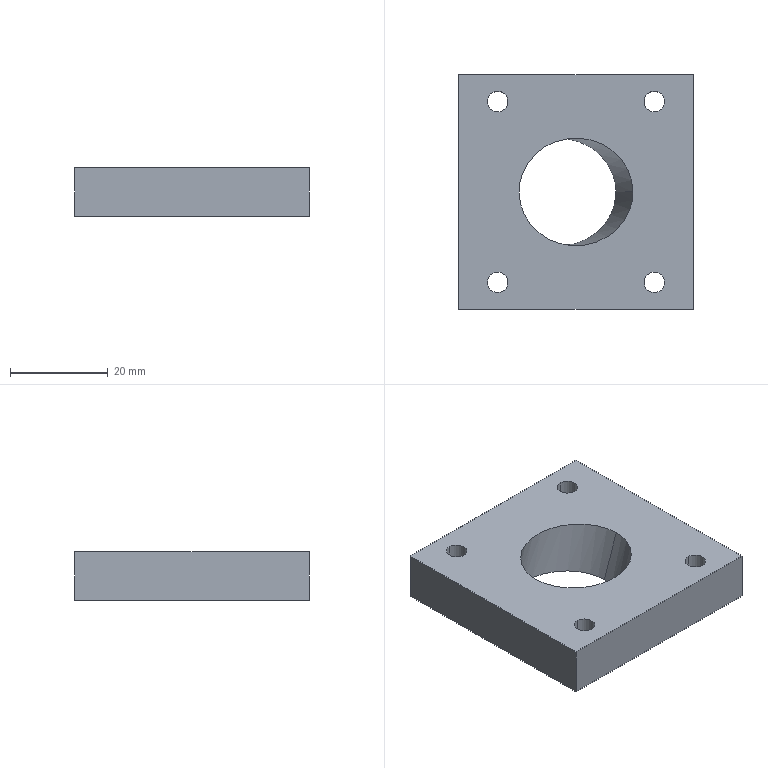Part | SolidWorks | features BaseBody 1 | 1 solid | 16 faces | box 48 x 48 x 10 mm | volume 18462 mm3 | cylinder 10 | plane 6 | commonest cylinder face diameters 4.2 x8 22 x2
STEP:
#1=CARTESIAN_POINT('',(-11.643,0.,10.));
#2=VERTEX_POINT('',#1);
#3=CARTESIAN_POINT('',(11.643,0.,10.));
#4=VERTEX_POINT('',#3);
#5=CARTESIAN_POINT('',(-11.643,0.,10.));
#6=CARTESIAN_POINT('',(-11.643,-22.,10.));
#7=CARTESIAN_POINT('',(11.643,-22.,10.));
#8=CARTESIAN_POINT('',(11.643,0.,10.));
#9=(BOUNDED_CURVE()B_SPLINE_CURVE(3,(#5,#6,#7,#8),.UNSPECIFIED.,.F.,.F.)B_SPLINE_CURVE_WITH_KNOTS((4,4),(0.,3.142),.UNSPECIFIED.)CURVE()GEOMETRIC_REPRESENTATION_ITEM()RATIONAL_B_SPLINE_CURVE((1.,0.3333,0.3333,1.))REPRESENTATION_ITEM(''));
#10=EDGE_CURVE('',#2,#4,#9,.T.);
#11=ORIENTED_EDGE('',*,*,#10,.T.);
#12=CARTESIAN_POINT('',(8.174,0.,0.));
#13=VERTEX_POINT('',#12);
#14=CARTESIAN_POINT('',(11.679,0.,10.103));
#15=DIRECTION('',(-0.3277,0.,-0.9448));
#16=VECTOR('',#15,1000.);
#17=LINE('',#14,#16);
#18=EDGE_CURVE('',#4,#13,#17,.T.);
#19=ORIENTED_EDGE('',*,*,#18,.T.);
#20=CARTESIAN_POINT('',(-15.112,0.,0.));
#21=VERTEX_POINT('',#20);
#22=CARTESIAN_POINT('',(8.174,0.,0.));
#23=CARTESIAN_POINT('',(8.174,-22.,0.));
#24=CARTESIAN_POINT('',(-15.112,-22.,0.));
#25=CARTESIAN_POINT('',(-15.112,0.,0.));
#26=(BOUNDED_CURVE()B_SPLINE_CURVE(3,(#22,#23,#24,#25),.UNSPECIFIED.,.F.,.F.)B_SPLINE_CURVE_WITH_KNOTS((4,4),(3.142,6.283),.UNSPECIFIED.)CURVE()GEOMETRIC_REPRESENTATION_ITEM()RATIONAL_B_SPLINE_CURVE((1.,0.3333,0.3333,1.))REPRESENTATION_ITEM(''));
#27=EDGE_CURVE('',#13,#21,#26,.T.);
#28=ORIENTED_EDGE('',*,*,#27,.T.);
#29=CARTESIAN_POINT('',(-9.106,0.,17.313));
#30=DIRECTION('',(-0.3277,0.,-0.9448));
#31=VECTOR('',#30,1000.);
#32=LINE('',#29,#31);
#33=EDGE_CURVE('',#2,#21,#32,.T.);
#34=ORIENTED_EDGE('',*,*,#33,.F.);
#35=EDGE_LOOP('',(#11,#19,#28,#34));
#36=FACE_OUTER_BOUND('',#35,.T.);
#37=CARTESIAN_POINT('',(1.286,0.,13.708));
#38=DIRECTION('',(-0.3277,0.,-0.9448));
#39=DIRECTION('',(-0.9448,0.,0.3277));
#40=AXIS2_PLACEMENT_3D('',#37,#38,#39);
#41=CYLINDRICAL_SURFACE('',#40,11.);
#42=ADVANCED_FACE('',(#36),#41,.F.);
#43=CARTESIAN_POINT('',(16.,20.6,10.));
#44=VERTEX_POINT('',#43);
#45=CARTESIAN_POINT('',(16.,16.4,10.));
#46=VERTEX_POINT('',#45);
#47=CARTESIAN_POINT('',(16.,18.5,10.));
#48=DIRECTION('',(0.,0.,1.));
#49=DIRECTION('',(0.,1.,0.));
#50=AXIS2_PLACEMENT_3D('',#47,#48,#49);
#51=CIRCLE('',#50,2.1);
#52=EDGE_CURVE('',#44,#46,#51,.T.);
#53=ORIENTED_EDGE('',*,*,#52,.T.);
#54=CARTESIAN_POINT('',(16.,16.4,0.));
#55=VERTEX_POINT('',#54);
#56=CARTESIAN_POINT('',(16.,16.4,10.));
#57=DIRECTION('',(0.,0.,-1.));
#58=VECTOR('',#57,1000.);
#59=LINE('',#56,#58);
#60=EDGE_CURVE('',#46,#55,#59,.T.);
#61=ORIENTED_EDGE('',*,*,#60,.T.);
#62=CARTESIAN_POINT('',(16.,20.6,0.));
#63=VERTEX_POINT('',#62);
#64=CARTESIAN_POINT('',(16.,18.5,0.));
#65=DIRECTION('',(0.,0.,1.));
#66=DIRECTION('',(0.,1.,0.));
#67=AXIS2_PLACEMENT_3D('',#64,#65,#66);
#68=CIRCLE('',#67,2.1);
#69=EDGE_CURVE('',#63,#55,#68,.T.);
#70=ORIENTED_EDGE('',*,*,#69,.F.);
#71=CARTESIAN_POINT('',(16.,20.6,10.));
#72=DIRECTION('',(0.,0.,-1.));
#73=VECTOR('',#72,1000.);
#74=LINE('',#71,#73);
#75=EDGE_CURVE('',#44,#63,#74,.T.);
#76=ORIENTED_EDGE('',*,*,#75,.F.);
#77=EDGE_LOOP('',(#53,#61,#70,#76));
#78=FACE_OUTER_BOUND('',#77,.T.);
#79=CARTESIAN_POINT('',(16.,18.5,10.));
#80=DIRECTION('',(0.,0.,-1.));
#81=DIRECTION('',(0.,1.,0.));
#82=AXIS2_PLACEMENT_3D('',#79,#80,#81);
#83=CYLINDRICAL_SURFACE('',#82,2.1);
#84=ADVANCED_FACE('',(#78),#83,.F.);
#85=CARTESIAN_POINT('',(-16.,-16.4,10.));
#86=VERTEX_POINT('',#85);
#87=CARTESIAN_POINT('',(-16.,-20.6,10.));
#88=VERTEX_POINT('',#87);
#89=CARTESIAN_POINT('',(-16.,-18.5,10.));
#90=DIRECTION('',(0.,0.,1.));
#91=DIRECTION('',(0.,1.,0.));
#92=AXIS2_PLACEMENT_3D('',#89,#90,#91);
#93=CIRCLE('',#92,2.1);
#94=EDGE_CURVE('',#86,#88,#93,.T.);
#95=ORIENTED_EDGE('',*,*,#94,.T.);
#96=CARTESIAN_POINT('',(-16.,-20.6,0.));
#97=VERTEX_POINT('',#96);
#98=CARTESIAN_POINT('',(-16.,-20.6,10.));
#99=DIRECTION('',(0.,0.,-1.));
#100=VECTOR('',#99,1000.);
#101=LINE('',#98,#100);
#102=EDGE_CURVE('',#88,#97,#101,.T.);
#103=ORIENTED_EDGE('',*,*,#102,.T.);
#104=CARTESIAN_POINT('',(-16.,-16.4,0.));
#105=VERTEX_POINT('',#104);
#106=CARTESIAN_POINT('',(-16.,-18.5,0.));
#107=DIRECTION('',(0.,0.,1.));
#108=DIRECTION('',(0.,1.,0.));
#109=AXIS2_PLACEMENT_3D('',#106,#107,#108);
#110=CIRCLE('',#109,2.1);
#111=EDGE_CURVE('',#105,#97,#110,.T.);
#112=ORIENTED_EDGE('',*,*,#111,.F.);
#113=CARTESIAN_POINT('',(-16.,-16.4,10.));
#114=DIRECTION('',(0.,0.,-1.));
#115=VECTOR('',#114,1000.);
#116=LINE('',#113,#115);
#117=EDGE_CURVE('',#86,#105,#116,.T.);
#118=ORIENTED_EDGE('',*,*,#117,.F.);
#119=EDGE_LOOP('',(#95,#103,#112,#118));
#120=FACE_OUTER_BOUND('',#119,.T.);
#121=CARTESIAN_POINT('',(-16.,-18.5,10.));
#122=DIRECTION('',(0.,0.,-1.));
#123=DIRECTION('',(0.,1.,0.));
#124=AXIS2_PLACEMENT_3D('',#121,#122,#123);
#125=CYLINDRICAL_SURFACE('',#124,2.1);
#126=ADVANCED_FACE('',(#120),#125,.F.);
#127=CARTESIAN_POINT('',(-16.,20.6,10.));
#128=VERTEX_POINT('',#127);
#129=CARTESIAN_POINT('',(-16.,16.4,10.));
#130=VERTEX_POINT('',#129);
#131=CARTESIAN_POINT('',(-16.,18.5,10.));
#132=DIRECTION('',(0.,0.,1.));
#133=DIRECTION('',(0.,1.,0.));
#134=AXIS2_PLACEMENT_3D('',#131,#132,#133);
#135=CIRCLE('',#134,2.1);
#136=EDGE_CURVE('',#128,#130,#135,.T.);
#137=ORIENTED_EDGE('',*,*,#136,.T.);
#138=CARTESIAN_POINT('',(-16.,16.4,0.));
#139=VERTEX_POINT('',#138);
#140=CARTESIAN_POINT('',(-16.,16.4,10.));
#141=DIRECTION('',(0.,0.,-1.));
#142=VECTOR('',#141,1000.);
#143=LINE('',#140,#142);
#144=EDGE_CURVE('',#130,#139,#143,.T.);
#145=ORIENTED_EDGE('',*,*,#144,.T.);
#146=CARTESIAN_POINT('',(-16.,20.6,0.));
#147=VERTEX_POINT('',#146);
#148=CARTESIAN_POINT('',(-16.,18.5,0.));
#149=DIRECTION('',(0.,0.,1.));
#150=DIRECTION('',(0.,1.,0.));
#151=AXIS2_PLACEMENT_3D('',#148,#149,#150);
#152=CIRCLE('',#151,2.1);
#153=EDGE_CURVE('',#147,#139,#152,.T.);
#154=ORIENTED_EDGE('',*,*,#153,.F.);
#155=CARTESIAN_POINT('',(-16.,20.6,10.));
#156=DIRECTION('',(0.,0.,-1.));
#157=VECTOR('',#156,1000.);
#158=LINE('',#155,#157);
#159=EDGE_CURVE('',#128,#147,#158,.T.);
#160=ORIENTED_EDGE('',*,*,#159,.F.);
#161=EDGE_LOOP('',(#137,#145,#154,#160));
#162=FACE_OUTER_BOUND('',#161,.T.);
#163=CARTESIAN_POINT('',(-16.,18.5,10.));
#164=DIRECTION('',(0.,0.,-1.));
#165=DIRECTION('',(0.,1.,0.));
#166=AXIS2_PLACEMENT_3D('',#163,#164,#165);
#167=CYLINDRICAL_SURFACE('',#166,2.1);
#168=ADVANCED_FACE('',(#162),#167,.F.);
#169=CARTESIAN_POINT('',(16.,-16.4,10.));
#170=VERTEX_POINT('',#169);
#171=CARTESIAN_POINT('',(16.,-20.6,10.));
#172=VERTEX_POINT('',#171);
#173=CARTESIAN_POINT('',(16.,-18.5,10.));
#174=DIRECTION('',(0.,0.,1.));
#175=DIRECTION('',(0.,1.,0.));
#176=AXIS2_PLACEMENT_3D('',#173,#174,#175);
#177=CIRCLE('',#176,2.1);
#178=EDGE_CURVE('',#170,#172,#177,.T.);
#179=ORIENTED_EDGE('',*,*,#178,.T.);
#180=CARTESIAN_POINT('',(16.,-20.6,0.));
#181=VERTEX_POINT('',#180);
#182=CARTESIAN_POINT('',(16.,-20.6,10.));
#183=DIRECTION('',(0.,0.,-1.));
#184=VECTOR('',#183,1000.);
#185=LINE('',#182,#184);
#186=EDGE_CURVE('',#172,#181,#185,.T.);
#187=ORIENTED_EDGE('',*,*,#186,.T.);
#188=CARTESIAN_POINT('',(16.,-16.4,0.));
#189=VERTEX_POINT('',#188);
#190=CARTESIAN_POINT('',(16.,-18.5,0.));
#191=DIRECTION('',(0.,0.,1.));
#192=DIRECTION('',(0.,1.,0.));
#193=AXIS2_PLACEMENT_3D('',#190,#191,#192);
#194=CIRCLE('',#193,2.1);
#195=EDGE_CURVE('',#189,#181,#194,.T.);
#196=ORIENTED_EDGE('',*,*,#195,.F.);
#197=CARTESIAN_POINT('',(16.,-16.4,10.));
#198=DIRECTION('',(0.,0.,-1.));
#199=VECTOR('',#198,1000.);
#200=LINE('',#197,#199);
#201=EDGE_CURVE('',#170,#189,#200,.T.);
#202=ORIENTED_EDGE('',*,*,#201,.F.);
#203=EDGE_LOOP('',(#179,#187,#196,#202));
#204=FACE_OUTER_BOUND('',#203,.T.);
#205=CARTESIAN_POINT('',(16.,-18.5,10.));
#206=DIRECTION('',(0.,0.,-1.));
#207=DIRECTION('',(0.,1.,0.));
#208=AXIS2_PLACEMENT_3D('',#205,#206,#207);
#209=CYLINDRICAL_SURFACE('',#208,2.1);
#210=ADVANCED_FACE('',(#204),#209,.F.);
#211=ORIENTED_EDGE('',*,*,#18,.F.);
#212=CARTESIAN_POINT('',(11.643,0.,10.));
#213=CARTESIAN_POINT('',(11.643,22.,10.));
#214=CARTESIAN_POINT('',(-11.643,22.,10.));
#215=CARTESIAN_POINT('',(-11.643,0.,10.));
#216=(BOUNDED_CURVE()B_SPLINE_CURVE(3,(#212,#213,#214,#215),.UNSPECIFIED.,.F.,.F.)B_SPLINE_CURVE_WITH_KNOTS((4,4),(3.142,6.283),.UNSPECIFIED.)CURVE()GEOMETRIC_REPRESENTATION_ITEM()RATIONAL_B_SPLINE_CURVE((1.,0.3333,0.3333,1.))REPRESENTATION_ITEM(''));
#217=EDGE_CURVE('',#4,#2,#216,.T.);
#218=ORIENTED_EDGE('',*,*,#217,.T.);
#219=ORIENTED_EDGE('',*,*,#33,.T.);
#220=CARTESIAN_POINT('',(-15.112,0.,0.));
#221=CARTESIAN_POINT('',(-15.112,22.,0.));
#222=CARTESIAN_POINT('',(8.174,22.,0.));
#223=CARTESIAN_POINT('',(8.174,0.,0.));
#224=(BOUNDED_CURVE()B_SPLINE_CURVE(3,(#220,#221,#222,#223),.UNSPECIFIED.,.F.,.F.)B_SPLINE_CURVE_WITH_KNOTS((4,4),(0.,3.142),.UNSPECIFIED.)CURVE()GEOMETRIC_REPRESENTATION_ITEM()RATIONAL_B_SPLINE_CURVE((1.,0.3333,0.3333,1.))REPRESENTATION_ITEM(''));
#225=EDGE_CURVE('',#21,#13,#224,.T.);
#226=ORIENTED_EDGE('',*,*,#225,.T.);
#227=EDGE_LOOP('',(#211,#218,#219,#226));
#228=FACE_OUTER_BOUND('',#227,.T.);
#229=CARTESIAN_POINT('',(1.286,0.,13.708));
#230=DIRECTION('',(-0.3277,0.,-0.9448));
#231=DIRECTION('',(-0.9448,0.,0.3277));
#232=AXIS2_PLACEMENT_3D('',#229,#230,#231);
#233=CYLINDRICAL_SURFACE('',#232,11.);
#234=ADVANCED_FACE('',(#228),#233,.F.);
#235=ORIENTED_EDGE('',*,*,#69,.T.);
#236=CARTESIAN_POINT('',(16.,18.5,0.));
#237=DIRECTION('',(0.,0.,1.));
#238=DIRECTION('',(0.,1.,0.));
#239=AXIS2_PLACEMENT_3D('',#236,#237,#238);
#240=CIRCLE('',#239,2.1);
#241=EDGE_CURVE('',#55,#63,#240,.T.);
#242=ORIENTED_EDGE('',*,*,#241,.T.);
#243=EDGE_LOOP('',(#235,#242));
#244=FACE_BOUND('',#243,.T.);
#245=ORIENTED_EDGE('',*,*,#111,.T.);
#246=CARTESIAN_POINT('',(-16.,-18.5,0.));
#247=DIRECTION('',(0.,0.,1.));
#248=DIRECTION('',(0.,1.,0.));
#249=AXIS2_PLACEMENT_3D('',#246,#247,#248);
#250=CIRCLE('',#249,2.1);
#251=EDGE_CURVE('',#97,#105,#250,.T.);
#252=ORIENTED_EDGE('',*,*,#251,.T.);
#253=EDGE_LOOP('',(#245,#252));
#254=FACE_BOUND('',#253,.T.);
#255=ORIENTED_EDGE('',*,*,#153,.T.);
#256=CARTESIAN_POINT('',(-16.,18.5,0.));
#257=DIRECTION('',(0.,0.,1.));
#258=DIRECTION('',(0.,1.,0.));
#259=AXIS2_PLACEMENT_3D('',#256,#257,#258);
#260=CIRCLE('',#259,2.1);
#261=EDGE_CURVE('',#139,#147,#260,.T.);
#262=ORIENTED_EDGE('',*,*,#261,.T.);
#263=EDGE_LOOP('',(#255,#262));
#264=FACE_BOUND('',#263,.T.);
#265=ORIENTED_EDGE('',*,*,#195,.T.);
#266=CARTESIAN_POINT('',(16.,-18.5,0.));
#267=DIRECTION('',(0.,0.,1.));
#268=DIRECTION('',(0.,1.,0.));
#269=AXIS2_PLACEMENT_3D('',#266,#267,#268);
#270=CIRCLE('',#269,2.1);
#271=EDGE_CURVE('',#181,#189,#270,.T.);
#272=ORIENTED_EDGE('',*,*,#271,.T.);
#273=EDGE_LOOP('',(#265,#272));
#274=FACE_BOUND('',#273,.T.);
#275=ORIENTED_EDGE('',*,*,#225,.F.);
#276=ORIENTED_EDGE('',*,*,#27,.F.);
#277=EDGE_LOOP('',(#275,#276));
#278=FACE_BOUND('',#277,.T.);
#279=CARTESIAN_POINT('',(24.,24.,0.));
#280=VERTEX_POINT('',#279);
#281=CARTESIAN_POINT('',(24.,-24.,0.));
#282=VERTEX_POINT('',#281);
#283=CARTESIAN_POINT('',(24.,0.,0.));
#284=DIRECTION('',(0.,-1.,0.));
#285=VECTOR('',#284,1000.);
#286=LINE('',#283,#285);
#287=EDGE_CURVE('',#280,#282,#286,.T.);
#288=ORIENTED_EDGE('',*,*,#287,.T.);
#289=CARTESIAN_POINT('',(-24.,-24.,0.));
#290=VERTEX_POINT('',#289);
#291=CARTESIAN_POINT('',(0.,-24.,0.));
#292=DIRECTION('',(-1.,0.,0.));
#293=VECTOR('',#292,1000.);
#294=LINE('',#291,#293);
#295=EDGE_CURVE('',#282,#290,#294,.T.);
#296=ORIENTED_EDGE('',*,*,#295,.T.);
#297=CARTESIAN_POINT('',(-24.,24.,0.));
#298=VERTEX_POINT('',#297);
#299=CARTESIAN_POINT('',(-24.,0.,0.));
#300=DIRECTION('',(0.,1.,0.));
#301=VECTOR('',#300,1000.);
#302=LINE('',#299,#301);
#303=EDGE_CURVE('',#290,#298,#302,.T.);
#304=ORIENTED_EDGE('',*,*,#303,.T.);
#305=CARTESIAN_POINT('',(0.,24.,0.));
#306=DIRECTION('',(1.,0.,0.));
#307=VECTOR('',#306,1000.);
#308=LINE('',#305,#307);
#309=EDGE_CURVE('',#298,#280,#308,.T.);
#310=ORIENTED_EDGE('',*,*,#309,.T.);
#311=EDGE_LOOP('',(#288,#296,#304,#310));
#312=FACE_OUTER_BOUND('',#311,.T.);
#313=CARTESIAN_POINT('',(24.,-24.,0.));
#314=DIRECTION('',(0.,0.,-1.));
#315=DIRECTION('',(-1.,0.,0.));
#316=AXIS2_PLACEMENT_3D('',#313,#314,#315);
#317=PLANE('',#316);
#318=ADVANCED_FACE('',(#244,#254,#264,#274,#278,#312),#317,.T.);
#319=ORIENTED_EDGE('',*,*,#52,.F.);
#320=CARTESIAN_POINT('',(16.,18.5,10.));
#321=DIRECTION('',(0.,0.,1.));
#322=DIRECTION('',(0.,1.,0.));
#323=AXIS2_PLACEMENT_3D('',#320,#321,#322);
#324=CIRCLE('',#323,2.1);
#325=EDGE_CURVE('',#46,#44,#324,.T.);
#326=ORIENTED_EDGE('',*,*,#325,.F.);
#327=EDGE_LOOP('',(#319,#326));
#328=FACE_BOUND('',#327,.T.);
#329=ORIENTED_EDGE('',*,*,#94,.F.);
#330=CARTESIAN_POINT('',(-16.,-18.5,10.));
#331=DIRECTION('',(0.,0.,1.));
#332=DIRECTION('',(0.,1.,0.));
#333=AXIS2_PLACEMENT_3D('',#330,#331,#332);
#334=CIRCLE('',#333,2.1);
#335=EDGE_CURVE('',#88,#86,#334,.T.);
#336=ORIENTED_EDGE('',*,*,#335,.F.);
#337=EDGE_LOOP('',(#329,#336));
#338=FACE_BOUND('',#337,.T.);
#339=ORIENTED_EDGE('',*,*,#136,.F.);
#340=CARTESIAN_POINT('',(-16.,18.5,10.));
#341=DIRECTION('',(0.,0.,1.));
#342=DIRECTION('',(0.,1.,0.));
#343=AXIS2_PLACEMENT_3D('',#340,#341,#342);
#344=CIRCLE('',#343,2.1);
#345=EDGE_CURVE('',#130,#128,#344,.T.);
#346=ORIENTED_EDGE('',*,*,#345,.F.);
#347=EDGE_LOOP('',(#339,#346));
#348=FACE_BOUND('',#347,.T.);
#349=ORIENTED_EDGE('',*,*,#178,.F.);
#350=CARTESIAN_POINT('',(16.,-18.5,10.));
#351=DIRECTION('',(0.,0.,1.));
#352=DIRECTION('',(0.,1.,0.));
#353=AXIS2_PLACEMENT_3D('',#350,#351,#352);
#354=CIRCLE('',#353,2.1);
#355=EDGE_CURVE('',#172,#170,#354,.T.);
#356=ORIENTED_EDGE('',*,*,#355,.F.);
#357=EDGE_LOOP('',(#349,#356));
#358=FACE_BOUND('',#357,.T.);
#359=ORIENTED_EDGE('',*,*,#10,.F.);
#360=ORIENTED_EDGE('',*,*,#217,.F.);
#361=EDGE_LOOP('',(#359,#360));
#362=FACE_BOUND('',#361,.T.);
#363=CARTESIAN_POINT('',(24.,-24.,10.));
#364=VERTEX_POINT('',#363);
#365=CARTESIAN_POINT('',(-24.,-24.,10.));
#366=VERTEX_POINT('',#365);
#367=CARTESIAN_POINT('',(0.,-24.,10.));
#368=DIRECTION('',(-1.,0.,0.));
#369=VECTOR('',#368,1000.);
#370=LINE('',#367,#369);
#371=EDGE_CURVE('',#364,#366,#370,.T.);
#372=ORIENTED_EDGE('',*,*,#371,.F.);
#373=CARTESIAN_POINT('',(24.,24.,10.));
#374=VERTEX_POINT('',#373);
#375=CARTESIAN_POINT('',(24.,0.,10.));
#376=DIRECTION('',(0.,-1.,0.));
#377=VECTOR('',#376,1000.);
#378=LINE('',#375,#377);
#379=EDGE_CURVE('',#374,#364,#378,.T.);
#380=ORIENTED_EDGE('',*,*,#379,.F.);
#381=CARTESIAN_POINT('',(-24.,24.,10.));
#382=VERTEX_POINT('',#381);
#383=CARTESIAN_POINT('',(0.,24.,10.));
#384=DIRECTION('',(1.,0.,0.));
#385=VECTOR('',#384,1000.);
#386=LINE('',#383,#385);
#387=EDGE_CURVE('',#382,#374,#386,.T.);
#388=ORIENTED_EDGE('',*,*,#387,.F.);
#389=CARTESIAN_POINT('',(-24.,0.,10.));
#390=DIRECTION('',(0.,1.,0.));
#391=VECTOR('',#390,1000.);
#392=LINE('',#389,#391);
#393=EDGE_CURVE('',#366,#382,#392,.T.);
#394=ORIENTED_EDGE('',*,*,#393,.F.);
#395=EDGE_LOOP('',(#372,#380,#388,#394));
#396=FACE_OUTER_BOUND('',#395,.T.);
#397=CARTESIAN_POINT('',(24.,-24.,10.));
#398=DIRECTION('',(0.,0.,-1.));
#399=DIRECTION('',(-1.,0.,0.));
#400=AXIS2_PLACEMENT_3D('',#397,#398,#399);
#401=PLANE('',#400);
#402=ADVANCED_FACE('',(#328,#338,#348,#358,#362,#396),#401,.F.);
#403=ORIENTED_EDGE('',*,*,#60,.F.);
#404=ORIENTED_EDGE('',*,*,#325,.T.);
#405=ORIENTED_EDGE('',*,*,#75,.T.);
#406=ORIENTED_EDGE('',*,*,#241,.F.);
#407=EDGE_LOOP('',(#403,#404,#405,#406));
#408=FACE_OUTER_BOUND('',#407,.T.);
#409=CARTESIAN_POINT('',(16.,18.5,10.));
#410=DIRECTION('',(0.,0.,-1.));
#411=DIRECTION('',(0.,1.,0.));
#412=AXIS2_PLACEMENT_3D('',#409,#410,#411);
#413=CYLINDRICAL_SURFACE('',#412,2.1);
#414=ADVANCED_FACE('',(#408),#413,.F.);
#415=ORIENTED_EDGE('',*,*,#102,.F.);
#416=ORIENTED_EDGE('',*,*,#335,.T.);
#417=ORIENTED_EDGE('',*,*,#117,.T.);
#418=ORIENTED_EDGE('',*,*,#251,.F.);
#419=EDGE_LOOP('',(#415,#416,#417,#418));
#420=FACE_OUTER_BOUND('',#419,.T.);
#421=CARTESIAN_POINT('',(-16.,-18.5,10.));
#422=DIRECTION('',(0.,0.,-1.));
#423=DIRECTION('',(0.,1.,0.));
#424=AXIS2_PLACEMENT_3D('',#421,#422,#423);
#425=CYLINDRICAL_SURFACE('',#424,2.1);
#426=ADVANCED_FACE('',(#420),#425,.F.);
#427=ORIENTED_EDGE('',*,*,#144,.F.);
#428=ORIENTED_EDGE('',*,*,#345,.T.);
#429=ORIENTED_EDGE('',*,*,#159,.T.);
#430=ORIENTED_EDGE('',*,*,#261,.F.);
#431=EDGE_LOOP('',(#427,#428,#429,#430));
#432=FACE_OUTER_BOUND('',#431,.T.);
#433=CARTESIAN_POINT('',(-16.,18.5,10.));
#434=DIRECTION('',(0.,0.,-1.));
#435=DIRECTION('',(0.,1.,0.));
#436=AXIS2_PLACEMENT_3D('',#433,#434,#435);
#437=CYLINDRICAL_SURFACE('',#436,2.1);
#438=ADVANCED_FACE('',(#432),#437,.F.);
#439=ORIENTED_EDGE('',*,*,#186,.F.);
#440=ORIENTED_EDGE('',*,*,#355,.T.);
#441=ORIENTED_EDGE('',*,*,#201,.T.);
#442=ORIENTED_EDGE('',*,*,#271,.F.);
#443=EDGE_LOOP('',(#439,#440,#441,#442));
#444=FACE_OUTER_BOUND('',#443,.T.);
#445=CARTESIAN_POINT('',(16.,-18.5,10.));
#446=DIRECTION('',(0.,0.,-1.));
#447=DIRECTION('',(0.,1.,0.));
#448=AXIS2_PLACEMENT_3D('',#445,#446,#447);
#449=CYLINDRICAL_SURFACE('',#448,2.1);
#450=ADVANCED_FACE('',(#444),#449,.F.);
#451=CARTESIAN_POINT('',(24.,-24.,5.));
#452=DIRECTION('',(0.,0.,-1.));
#453=VECTOR('',#452,1000.);
#454=LINE('',#451,#453);
#455=EDGE_CURVE('',#364,#282,#454,.T.);
#456=ORIENTED_EDGE('',*,*,#455,.F.);
#457=ORIENTED_EDGE('',*,*,#371,.T.);
#458=CARTESIAN_POINT('',(-24.,-24.,5.));
#459=DIRECTION('',(0.,0.,1.));
#460=VECTOR('',#459,1000.);
#461=LINE('',#458,#460);
#462=EDGE_CURVE('',#290,#366,#461,.T.);
#463=ORIENTED_EDGE('',*,*,#462,.F.);
#464=ORIENTED_EDGE('',*,*,#295,.F.);
#465=EDGE_LOOP('',(#456,#457,#463,#464));
#466=FACE_OUTER_BOUND('',#465,.T.);
#467=CARTESIAN_POINT('',(24.,-24.,0.));
#468=DIRECTION('',(0.,1.,0.));
#469=DIRECTION('',(-1.,0.,0.));
#470=AXIS2_PLACEMENT_3D('',#467,#468,#469);
#471=PLANE('',#470);
#472=ADVANCED_FACE('',(#466),#471,.F.);
#473=CARTESIAN_POINT('',(24.,24.,5.));
#474=DIRECTION('',(0.,0.,-1.));
#475=VECTOR('',#474,1000.);
#476=LINE('',#473,#475);
#477=EDGE_CURVE('',#374,#280,#476,.T.);
#478=ORIENTED_EDGE('',*,*,#477,.F.);
#479=ORIENTED_EDGE('',*,*,#379,.T.);
#480=ORIENTED_EDGE('',*,*,#455,.T.);
#481=ORIENTED_EDGE('',*,*,#287,.F.);
#482=EDGE_LOOP('',(#478,#479,#480,#481));
#483=FACE_OUTER_BOUND('',#482,.T.);
#484=CARTESIAN_POINT('',(24.,24.,0.));
#485=DIRECTION('',(-1.,0.,0.));
#486=DIRECTION('',(0.,-1.,0.));
#487=AXIS2_PLACEMENT_3D('',#484,#485,#486);
#488=PLANE('',#487);
#489=ADVANCED_FACE('',(#483),#488,.F.);
#490=CARTESIAN_POINT('',(-24.,24.,5.));
#491=DIRECTION('',(0.,0.,-1.));
#492=VECTOR('',#491,1000.);
#493=LINE('',#490,#492);
#494=EDGE_CURVE('',#382,#298,#493,.T.);
#495=ORIENTED_EDGE('',*,*,#494,.F.);
#496=ORIENTED_EDGE('',*,*,#387,.T.);
#497=ORIENTED_EDGE('',*,*,#477,.T.);
#498=ORIENTED_EDGE('',*,*,#309,.F.);
#499=EDGE_LOOP('',(#495,#496,#497,#498));
#500=FACE_OUTER_BOUND('',#499,.T.);
#501=CARTESIAN_POINT('',(-24.,24.,0.));
#502=DIRECTION('',(0.,-1.,0.));
#503=DIRECTION('',(1.,0.,0.));
#504=AXIS2_PLACEMENT_3D('',#501,#502,#503);
#505=PLANE('',#504);
#506=ADVANCED_FACE('',(#500),#505,.F.);
#507=ORIENTED_EDGE('',*,*,#462,.T.);
#508=ORIENTED_EDGE('',*,*,#393,.T.);
#509=ORIENTED_EDGE('',*,*,#494,.T.);
#510=ORIENTED_EDGE('',*,*,#303,.F.);
#511=EDGE_LOOP('',(#507,#508,#509,#510));
#512=FACE_OUTER_BOUND('',#511,.T.);
#513=CARTESIAN_POINT('',(-24.,-24.,0.));
#514=DIRECTION('',(1.,0.,0.));
#515=DIRECTION('',(0.,1.,0.));
#516=AXIS2_PLACEMENT_3D('',#513,#514,#515);
#517=PLANE('',#516);
#518=ADVANCED_FACE('',(#512),#517,.F.);
#519=CLOSED_SHELL('',(#42,#84,#126,#168,#210,#234,#318,#402,#414,#426,#438,#450,#472,#489,#506,#518));
#520=MANIFOLD_SOLID_BREP('',#519);
#521=CARTESIAN_POINT('',(0.,0.,0.));
#522=DIRECTION('',(0.,0.,1.));
#523=DIRECTION('',(1.,0.,0.));
#524=AXIS2_PLACEMENT_3D('',#521,#522,#523);
#525=(LENGTH_UNIT()NAMED_UNIT(*)SI_UNIT(.MILLI.,.METRE.));
#526=UNCERTAINTY_MEASURE_WITH_UNIT(LENGTH_MEASURE(0.00001),#525,'','');
#527=(NAMED_UNIT(*)PLANE_ANGLE_UNIT()SI_UNIT($,.RADIAN.));
#528=(NAMED_UNIT(*)SI_UNIT($,.STERADIAN.)SOLID_ANGLE_UNIT());
#529=(GEOMETRIC_REPRESENTATION_CONTEXT(3)GLOBAL_UNCERTAINTY_ASSIGNED_CONTEXT((#526))GLOBAL_UNIT_ASSIGNED_CONTEXT((#525,#527,#528))REPRESENTATION_CONTEXT('',''));
#530=ADVANCED_BREP_SHAPE_REPRESENTATION('',(#520,#524),#529);